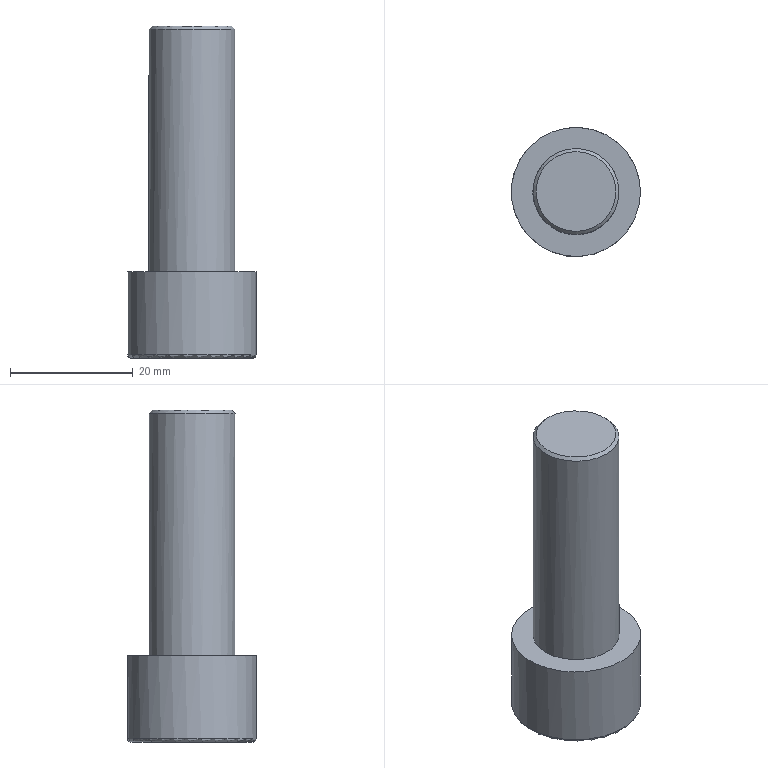Part | NX | features 模具.stp<1>[25] 2 | 1 solid | 14 faces | box 21 x 21 x 54 mm | volume 10125 mm3 | plane 10 | cylinder 2 | cone 1 | torus 1 | commonest cylinder face diameters 14 x1 21 x1
STEP:
#1=CARTESIAN_POINT('',(256.928,297.,-277.5));
#2=VERTEX_POINT('',#1);
#3=CARTESIAN_POINT('',(253.464,291.,-277.5));
#4=VERTEX_POINT('',#3);
#5=CARTESIAN_POINT('',(256.928,297.,-277.5));
#6=DIRECTION('',(-0.5,-0.866,0.));
#7=VECTOR('',#6,1000.);
#8=LINE('',#5,#7);
#9=EDGE_CURVE('',#2,#4,#8,.T.);
#10=ORIENTED_EDGE('',*,*,#9,.T.);
#11=CARTESIAN_POINT('',(246.536,291.,-277.5));
#12=VERTEX_POINT('',#11);
#13=CARTESIAN_POINT('',(253.464,291.,-277.5));
#14=DIRECTION('',(-1.,0.,0.));
#15=VECTOR('',#14,1000.);
#16=LINE('',#13,#15);
#17=EDGE_CURVE('',#4,#12,#16,.T.);
#18=ORIENTED_EDGE('',*,*,#17,.T.);
#19=CARTESIAN_POINT('',(243.072,297.,-277.5));
#20=VERTEX_POINT('',#19);
#21=CARTESIAN_POINT('',(246.536,291.,-277.5));
#22=DIRECTION('',(-0.5,0.866,0.));
#23=VECTOR('',#22,1000.);
#24=LINE('',#21,#23);
#25=EDGE_CURVE('',#12,#20,#24,.T.);
#26=ORIENTED_EDGE('',*,*,#25,.T.);
#27=CARTESIAN_POINT('',(246.536,303.,-277.5));
#28=VERTEX_POINT('',#27);
#29=CARTESIAN_POINT('',(243.072,297.,-277.5));
#30=DIRECTION('',(0.5,0.866,0.));
#31=VECTOR('',#30,1000.);
#32=LINE('',#29,#31);
#33=EDGE_CURVE('',#20,#28,#32,.T.);
#34=ORIENTED_EDGE('',*,*,#33,.T.);
#35=CARTESIAN_POINT('',(253.464,303.,-277.5));
#36=VERTEX_POINT('',#35);
#37=CARTESIAN_POINT('',(246.536,303.,-277.5));
#38=DIRECTION('',(1.,0.,0.));
#39=VECTOR('',#38,1000.);
#40=LINE('',#37,#39);
#41=EDGE_CURVE('',#28,#36,#40,.T.);
#42=ORIENTED_EDGE('',*,*,#41,.T.);
#43=CARTESIAN_POINT('',(253.464,303.,-277.5));
#44=DIRECTION('',(0.5,-0.866,0.));
#45=VECTOR('',#44,1000.);
#46=LINE('',#43,#45);
#47=EDGE_CURVE('',#36,#2,#46,.T.);
#48=ORIENTED_EDGE('',*,*,#47,.T.);
#49=EDGE_LOOP('',(#10,#18,#26,#34,#42,#48));
#50=FACE_BOUND('',#49,.T.);
#51=CARTESIAN_POINT('',(250.,297.,-277.5));
#52=DIRECTION('',(0.,0.,1.));
#53=DIRECTION('',(0.,-1.,0.));
#54=AXIS2_PLACEMENT_3D('',#51,#52,#53);
#55=PLANE('',#54);
#56=ADVANCED_FACE('',(#50),#55,.F.);
#57=CARTESIAN_POINT('',(256.928,297.,-284.5));
#58=VERTEX_POINT('',#57);
#59=CARTESIAN_POINT('',(253.464,291.,-284.5));
#60=VERTEX_POINT('',#59);
#61=CARTESIAN_POINT('',(256.928,297.,-284.5));
#62=DIRECTION('',(-0.5,-0.866,0.));
#63=VECTOR('',#62,1000.);
#64=LINE('',#61,#63);
#65=EDGE_CURVE('',#58,#60,#64,.T.);
#66=ORIENTED_EDGE('',*,*,#65,.T.);
#67=CARTESIAN_POINT('',(253.464,291.,-277.5));
#68=DIRECTION('',(0.,0.,-1.));
#69=VECTOR('',#68,1000.);
#70=LINE('',#67,#69);
#71=EDGE_CURVE('',#4,#60,#70,.T.);
#72=ORIENTED_EDGE('',*,*,#71,.F.);
#73=ORIENTED_EDGE('',*,*,#9,.F.);
#74=CARTESIAN_POINT('',(256.928,297.,-277.5));
#75=DIRECTION('',(0.,0.,-1.));
#76=VECTOR('',#75,1000.);
#77=LINE('',#74,#76);
#78=EDGE_CURVE('',#2,#58,#77,.T.);
#79=ORIENTED_EDGE('',*,*,#78,.T.);
#80=EDGE_LOOP('',(#66,#72,#73,#79));
#81=FACE_BOUND('',#80,.T.);
#82=CARTESIAN_POINT('',(255.196,294.,-281.));
#83=DIRECTION('',(0.866,-0.5,0.));
#84=DIRECTION('',(0.,0.,-1.));
#85=AXIS2_PLACEMENT_3D('',#82,#83,#84);
#86=PLANE('',#85);
#87=ADVANCED_FACE('',(#81),#86,.F.);
#88=CARTESIAN_POINT('',(246.536,291.,-284.5));
#89=VERTEX_POINT('',#88);
#90=CARTESIAN_POINT('',(253.464,291.,-284.5));
#91=DIRECTION('',(-1.,0.,0.));
#92=VECTOR('',#91,1000.);
#93=LINE('',#90,#92);
#94=EDGE_CURVE('',#60,#89,#93,.T.);
#95=ORIENTED_EDGE('',*,*,#94,.T.);
#96=CARTESIAN_POINT('',(246.536,291.,-277.5));
#97=DIRECTION('',(0.,0.,-1.));
#98=VECTOR('',#97,1000.);
#99=LINE('',#96,#98);
#100=EDGE_CURVE('',#12,#89,#99,.T.);
#101=ORIENTED_EDGE('',*,*,#100,.F.);
#102=ORIENTED_EDGE('',*,*,#17,.F.);
#103=ORIENTED_EDGE('',*,*,#71,.T.);
#104=EDGE_LOOP('',(#95,#101,#102,#103));
#105=FACE_BOUND('',#104,.T.);
#106=CARTESIAN_POINT('',(250.,291.,-281.));
#107=DIRECTION('',(0.,-1.,0.));
#108=DIRECTION('',(0.,0.,-1.));
#109=AXIS2_PLACEMENT_3D('',#106,#107,#108);
#110=PLANE('',#109);
#111=ADVANCED_FACE('',(#105),#110,.F.);
#112=CARTESIAN_POINT('',(243.072,297.,-284.5));
#113=VERTEX_POINT('',#112);
#114=CARTESIAN_POINT('',(246.536,291.,-284.5));
#115=DIRECTION('',(-0.5,0.866,0.));
#116=VECTOR('',#115,1000.);
#117=LINE('',#114,#116);
#118=EDGE_CURVE('',#89,#113,#117,.T.);
#119=ORIENTED_EDGE('',*,*,#118,.T.);
#120=CARTESIAN_POINT('',(243.072,297.,-277.5));
#121=DIRECTION('',(0.,0.,-1.));
#122=VECTOR('',#121,1000.);
#123=LINE('',#120,#122);
#124=EDGE_CURVE('',#20,#113,#123,.T.);
#125=ORIENTED_EDGE('',*,*,#124,.F.);
#126=ORIENTED_EDGE('',*,*,#25,.F.);
#127=ORIENTED_EDGE('',*,*,#100,.T.);
#128=EDGE_LOOP('',(#119,#125,#126,#127));
#129=FACE_BOUND('',#128,.T.);
#130=CARTESIAN_POINT('',(244.804,294.,-281.));
#131=DIRECTION('',(-0.866,-0.5,0.));
#132=DIRECTION('',(-0.5,0.866,0.));
#133=AXIS2_PLACEMENT_3D('',#130,#131,#132);
#134=PLANE('',#133);
#135=ADVANCED_FACE('',(#129),#134,.F.);
#136=CARTESIAN_POINT('',(246.536,303.,-284.5));
#137=VERTEX_POINT('',#136);
#138=CARTESIAN_POINT('',(243.072,297.,-284.5));
#139=DIRECTION('',(0.5,0.866,0.));
#140=VECTOR('',#139,1000.);
#141=LINE('',#138,#140);
#142=EDGE_CURVE('',#113,#137,#141,.T.);
#143=ORIENTED_EDGE('',*,*,#142,.T.);
#144=CARTESIAN_POINT('',(246.536,303.,-277.5));
#145=DIRECTION('',(0.,0.,-1.));
#146=VECTOR('',#145,1000.);
#147=LINE('',#144,#146);
#148=EDGE_CURVE('',#28,#137,#147,.T.);
#149=ORIENTED_EDGE('',*,*,#148,.F.);
#150=ORIENTED_EDGE('',*,*,#33,.F.);
#151=ORIENTED_EDGE('',*,*,#124,.T.);
#152=EDGE_LOOP('',(#143,#149,#150,#151));
#153=FACE_BOUND('',#152,.T.);
#154=CARTESIAN_POINT('',(244.804,300.,-281.));
#155=DIRECTION('',(-0.866,0.5,0.));
#156=DIRECTION('',(0.,0.,1.));
#157=AXIS2_PLACEMENT_3D('',#154,#155,#156);
#158=PLANE('',#157);
#159=ADVANCED_FACE('',(#153),#158,.F.);
#160=CARTESIAN_POINT('',(253.464,303.,-284.5));
#161=VERTEX_POINT('',#160);
#162=CARTESIAN_POINT('',(246.536,303.,-284.5));
#163=DIRECTION('',(1.,0.,0.));
#164=VECTOR('',#163,1000.);
#165=LINE('',#162,#164);
#166=EDGE_CURVE('',#137,#161,#165,.T.);
#167=ORIENTED_EDGE('',*,*,#166,.T.);
#168=CARTESIAN_POINT('',(253.464,303.,-277.5));
#169=DIRECTION('',(0.,0.,-1.));
#170=VECTOR('',#169,1000.);
#171=LINE('',#168,#170);
#172=EDGE_CURVE('',#36,#161,#171,.T.);
#173=ORIENTED_EDGE('',*,*,#172,.F.);
#174=ORIENTED_EDGE('',*,*,#41,.F.);
#175=ORIENTED_EDGE('',*,*,#148,.T.);
#176=EDGE_LOOP('',(#167,#173,#174,#175));
#177=FACE_BOUND('',#176,.T.);
#178=CARTESIAN_POINT('',(250.,303.,-281.));
#179=DIRECTION('',(0.,1.,0.));
#180=DIRECTION('',(0.,0.,-1.));
#181=AXIS2_PLACEMENT_3D('',#178,#179,#180);
#182=PLANE('',#181);
#183=ADVANCED_FACE('',(#177),#182,.F.);
#184=CARTESIAN_POINT('',(253.464,303.,-284.5));
#185=DIRECTION('',(0.5,-0.866,0.));
#186=VECTOR('',#185,1000.);
#187=LINE('',#184,#186);
#188=EDGE_CURVE('',#161,#58,#187,.T.);
#189=ORIENTED_EDGE('',*,*,#188,.T.);
#190=ORIENTED_EDGE('',*,*,#78,.F.);
#191=ORIENTED_EDGE('',*,*,#47,.F.);
#192=ORIENTED_EDGE('',*,*,#172,.T.);
#193=EDGE_LOOP('',(#189,#190,#191,#192));
#194=FACE_BOUND('',#193,.T.);
#195=CARTESIAN_POINT('',(255.196,300.,-281.));
#196=DIRECTION('',(0.866,0.5,0.));
#197=DIRECTION('',(0.,0.,-1.));
#198=AXIS2_PLACEMENT_3D('',#195,#196,#197);
#199=PLANE('',#198);
#200=ADVANCED_FACE('',(#194),#199,.F.);
#201=CARTESIAN_POINT('',(257.,297.,-231.));
#202=VERTEX_POINT('',#201);
#203=CARTESIAN_POINT('',(250.,297.,-231.));
#204=DIRECTION('',(0.,0.,-1.));
#205=DIRECTION('',(1.,0.,0.));
#206=AXIS2_PLACEMENT_3D('',#203,#204,#205);
#207=CIRCLE('',#206,7.);
#208=EDGE_CURVE('',#202,#202,#207,.T.);
#209=ORIENTED_EDGE('',*,*,#208,.F.);
#210=EDGE_LOOP('',(#209));
#211=FACE_BOUND('',#210,.T.);
#212=CARTESIAN_POINT('',(250.,290.5,-230.5));
#213=VERTEX_POINT('',#212);
#214=CARTESIAN_POINT('',(250.,297.,-230.5));
#215=DIRECTION('',(0.,0.,1.));
#216=DIRECTION('',(0.,-1.,0.));
#217=AXIS2_PLACEMENT_3D('',#214,#215,#216);
#218=CIRCLE('',#217,6.5);
#219=EDGE_CURVE('',#213,#213,#218,.T.);
#220=ORIENTED_EDGE('',*,*,#219,.F.);
#221=EDGE_LOOP('',(#220));
#222=FACE_BOUND('',#221,.T.);
#223=CARTESIAN_POINT('',(250.,297.,-231.));
#224=DIRECTION('',(0.,0.,-1.));
#225=DIRECTION('',(-1.,0.,0.));
#226=AXIS2_PLACEMENT_3D('',#223,#224,#225);
#227=CONICAL_SURFACE('',#226,7.,0.7854);
#228=ADVANCED_FACE('',(#211,#222),#227,.T.);
#229=CARTESIAN_POINT('',(257.,297.,-270.5));
#230=VERTEX_POINT('',#229);
#231=CARTESIAN_POINT('',(250.,297.,-270.5));
#232=DIRECTION('',(0.,0.,1.));
#233=DIRECTION('',(1.,0.,0.));
#234=AXIS2_PLACEMENT_3D('',#231,#232,#233);
#235=CIRCLE('',#234,7.);
#236=EDGE_CURVE('',#230,#230,#235,.T.);
#237=ORIENTED_EDGE('',*,*,#236,.T.);
#238=EDGE_LOOP('',(#237));
#239=FACE_BOUND('',#238,.T.);
#240=ORIENTED_EDGE('',*,*,#208,.T.);
#241=EDGE_LOOP('',(#240));
#242=FACE_BOUND('',#241,.T.);
#243=CARTESIAN_POINT('',(250.,297.,-230.5));
#244=DIRECTION('',(0.,0.,-1.));
#245=DIRECTION('',(1.,0.,0.));
#246=AXIS2_PLACEMENT_3D('',#243,#244,#245);
#247=CYLINDRICAL_SURFACE('',#246,7.);
#248=ADVANCED_FACE('',(#239,#242),#247,.T.);
#249=ORIENTED_EDGE('',*,*,#219,.T.);
#250=EDGE_LOOP('',(#249));
#251=FACE_BOUND('',#250,.T.);
#252=CARTESIAN_POINT('',(250.,297.,-230.5));
#253=DIRECTION('',(0.,0.,1.));
#254=DIRECTION('',(0.,-1.,0.));
#255=AXIS2_PLACEMENT_3D('',#252,#253,#254);
#256=PLANE('',#255);
#257=ADVANCED_FACE('',(#251),#256,.T.);
#258=CARTESIAN_POINT('',(250.,307.5,-284.));
#259=VERTEX_POINT('',#258);
#260=CARTESIAN_POINT('',(250.,297.,-284.));
#261=DIRECTION('',(0.,0.,1.));
#262=DIRECTION('',(0.,1.,0.));
#263=AXIS2_PLACEMENT_3D('',#260,#261,#262);
#264=CIRCLE('',#263,10.5);
#265=EDGE_CURVE('',#259,#259,#264,.T.);
#266=ORIENTED_EDGE('',*,*,#265,.F.);
#267=EDGE_LOOP('',(#266));
#268=FACE_BOUND('',#267,.T.);
#269=CARTESIAN_POINT('',(250.,307.,-284.5));
#270=VERTEX_POINT('',#269);
#271=CARTESIAN_POINT('',(250.,297.,-284.5));
#272=DIRECTION('',(0.,0.,-1.));
#273=DIRECTION('',(0.,1.,0.));
#274=AXIS2_PLACEMENT_3D('',#271,#272,#273);
#275=CIRCLE('',#274,10.);
#276=EDGE_CURVE('',#270,#270,#275,.T.);
#277=ORIENTED_EDGE('',*,*,#276,.F.);
#278=EDGE_LOOP('',(#277));
#279=FACE_BOUND('',#278,.T.);
#280=CARTESIAN_POINT('',(250.,297.,-284.));
#281=DIRECTION('',(0.,0.,-1.));
#282=DIRECTION('',(0.,1.,0.));
#283=AXIS2_PLACEMENT_3D('',#280,#281,#282);
#284=TOROIDAL_SURFACE('',#283,10.,0.5);
#285=ADVANCED_FACE('',(#268,#279),#284,.T.);
#286=CARTESIAN_POINT('',(260.5,297.,-270.5));
#287=VERTEX_POINT('',#286);
#288=CARTESIAN_POINT('',(250.,297.,-270.5));
#289=DIRECTION('',(0.,0.,-1.));
#290=DIRECTION('',(1.,0.,0.));
#291=AXIS2_PLACEMENT_3D('',#288,#289,#290);
#292=CIRCLE('',#291,10.5);
#293=EDGE_CURVE('',#287,#287,#292,.T.);
#294=ORIENTED_EDGE('',*,*,#293,.T.);
#295=EDGE_LOOP('',(#294));
#296=FACE_BOUND('',#295,.T.);
#297=ORIENTED_EDGE('',*,*,#265,.T.);
#298=EDGE_LOOP('',(#297));
#299=FACE_BOUND('',#298,.T.);
#300=CARTESIAN_POINT('',(250.,297.,-270.5));
#301=DIRECTION('',(0.,0.,-1.));
#302=DIRECTION('',(1.,0.,0.));
#303=AXIS2_PLACEMENT_3D('',#300,#301,#302);
#304=CYLINDRICAL_SURFACE('',#303,10.5);
#305=ADVANCED_FACE('',(#296,#299),#304,.T.);
#306=ORIENTED_EDGE('',*,*,#293,.F.);
#307=EDGE_LOOP('',(#306));
#308=FACE_BOUND('',#307,.T.);
#309=ORIENTED_EDGE('',*,*,#236,.F.);
#310=EDGE_LOOP('',(#309));
#311=FACE_BOUND('',#310,.T.);
#312=CARTESIAN_POINT('',(250.,297.,-270.5));
#313=DIRECTION('',(0.,0.,1.));
#314=DIRECTION('',(0.,-1.,0.));
#315=AXIS2_PLACEMENT_3D('',#312,#313,#314);
#316=PLANE('',#315);
#317=ADVANCED_FACE('',(#308,#311),#316,.T.);
#318=ORIENTED_EDGE('',*,*,#276,.T.);
#319=EDGE_LOOP('',(#318));
#320=FACE_BOUND('',#319,.T.);
#321=ORIENTED_EDGE('',*,*,#188,.F.);
#322=ORIENTED_EDGE('',*,*,#166,.F.);
#323=ORIENTED_EDGE('',*,*,#142,.F.);
#324=ORIENTED_EDGE('',*,*,#118,.F.);
#325=ORIENTED_EDGE('',*,*,#94,.F.);
#326=ORIENTED_EDGE('',*,*,#65,.F.);
#327=EDGE_LOOP('',(#321,#322,#323,#324,#325,#326));
#328=FACE_BOUND('',#327,.T.);
#329=CARTESIAN_POINT('',(250.,297.,-284.5));
#330=DIRECTION('',(0.,0.,-1.));
#331=DIRECTION('',(0.,-1.,0.));
#332=AXIS2_PLACEMENT_3D('',#329,#330,#331);
#333=PLANE('',#332);
#334=ADVANCED_FACE('',(#320,#328),#333,.T.);
#335=CLOSED_SHELL('',(#56,#87,#111,#135,#159,#183,#200,#228,#248,#257,#285,#305,#317,#334));
#336=MANIFOLD_SOLID_BREP('',#335);
#337=(LENGTH_UNIT()NAMED_UNIT(*)SI_UNIT(.MILLI.,.METRE.));
#338=UNCERTAINTY_MEASURE_WITH_UNIT(LENGTH_MEASURE(0.00001),#337,'','');
#339=(NAMED_UNIT(*)PLANE_ANGLE_UNIT()SI_UNIT($,.RADIAN.));
#340=(NAMED_UNIT(*)SI_UNIT($,.STERADIAN.)SOLID_ANGLE_UNIT());
#341=(GEOMETRIC_REPRESENTATION_CONTEXT(3)GLOBAL_UNCERTAINTY_ASSIGNED_CONTEXT((#338))GLOBAL_UNIT_ASSIGNED_CONTEXT((#337,#339,#340))REPRESENTATION_CONTEXT('',''));
#342=ADVANCED_BREP_SHAPE_REPRESENTATION('',(#336),#341);